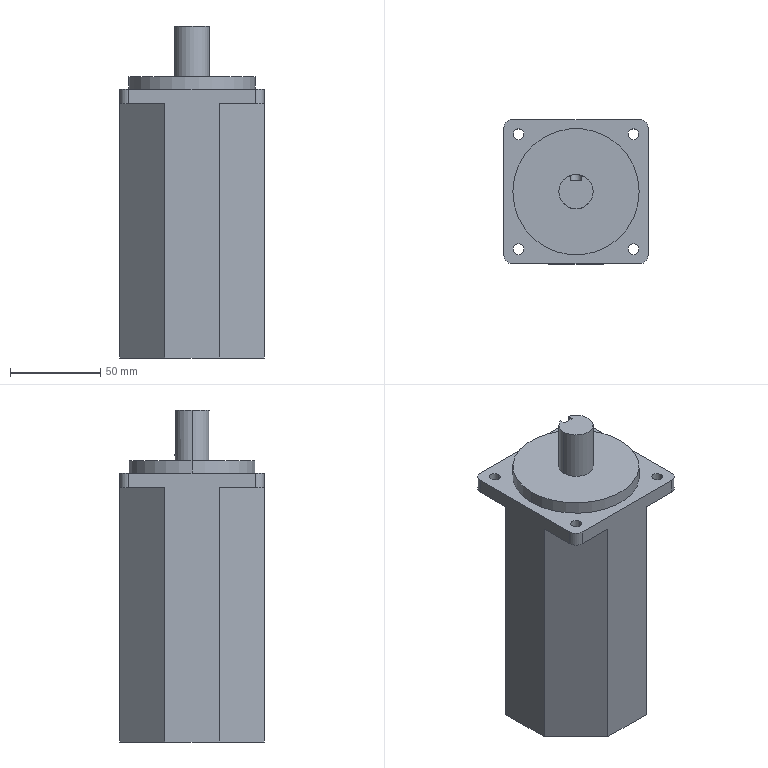Part | SolidWorks | features ICE 6, CombineBodies 1, Extrusion 1, Fillet 1 | 1 solid | 36 faces | box 80 x 80 x 184 mm | volume 810663 mm3 | plane 19 | cylinder 17 | commonest cylinder face diameters 6 x9 10 x4 19 x2 70 x2
STEP:
#1=CARTESIAN_POINT('',(49.5,40.,184.));
#2=VERTEX_POINT('',#1);
#3=CARTESIAN_POINT('',(43.,49.014,184.));
#4=VERTEX_POINT('',#3);
#5=CARTESIAN_POINT('',(40.,40.,184.));
#6=DIRECTION('',(0.,0.,1.));
#7=DIRECTION('',(1.,0.,0.));
#8=AXIS2_PLACEMENT_3D('',#5,#6,#7);
#9=CIRCLE('',#8,9.5);
#10=EDGE_CURVE('',#2,#4,#9,.T.);
#11=ORIENTED_EDGE('',*,*,#10,.F.);
#12=CARTESIAN_POINT('',(49.5,40.,156.));
#13=VERTEX_POINT('',#12);
#14=CARTESIAN_POINT('',(49.5,40.,184.));
#15=DIRECTION('',(0.,0.,-1.));
#16=VECTOR('',#15,1000.);
#17=LINE('',#14,#16);
#18=EDGE_CURVE('',#2,#13,#17,.T.);
#19=ORIENTED_EDGE('',*,*,#18,.T.);
#20=CARTESIAN_POINT('',(30.5,40.,156.));
#21=VERTEX_POINT('',#20);
#22=CARTESIAN_POINT('',(40.,40.,156.));
#23=DIRECTION('',(0.,0.,1.));
#24=DIRECTION('',(1.,0.,0.));
#25=AXIS2_PLACEMENT_3D('',#22,#23,#24);
#26=CIRCLE('',#25,9.5);
#27=EDGE_CURVE('',#13,#21,#26,.T.);
#28=ORIENTED_EDGE('',*,*,#27,.T.);
#29=CARTESIAN_POINT('',(30.5,40.,184.));
#30=VERTEX_POINT('',#29);
#31=CARTESIAN_POINT('',(30.5,40.,184.));
#32=DIRECTION('',(0.,0.,-1.));
#33=VECTOR('',#32,1000.);
#34=LINE('',#31,#33);
#35=EDGE_CURVE('',#30,#21,#34,.T.);
#36=ORIENTED_EDGE('',*,*,#35,.F.);
#37=CARTESIAN_POINT('',(37.,49.014,184.));
#38=VERTEX_POINT('',#37);
#39=CARTESIAN_POINT('',(40.,40.,184.));
#40=DIRECTION('',(0.,0.,1.));
#41=DIRECTION('',(1.,0.,0.));
#42=AXIS2_PLACEMENT_3D('',#39,#40,#41);
#43=CIRCLE('',#42,9.5);
#44=EDGE_CURVE('',#38,#30,#43,.T.);
#45=ORIENTED_EDGE('',*,*,#44,.F.);
#46=CARTESIAN_POINT('',(37.,49.014,162.));
#47=VERTEX_POINT('',#46);
#48=CARTESIAN_POINT('',(37.,49.014,184.));
#49=DIRECTION('',(0.,0.,-1.));
#50=VECTOR('',#49,1000.);
#51=LINE('',#48,#50);
#52=EDGE_CURVE('',#38,#47,#51,.T.);
#53=ORIENTED_EDGE('',*,*,#52,.T.);
#54=CARTESIAN_POINT('',(43.,49.014,162.));
#55=VERTEX_POINT('',#54);
#56=CARTESIAN_POINT('',(37.,49.014,162.));
#57=CARTESIAN_POINT('',(37.,49.014,161.803));
#58=CARTESIAN_POINT('',(37.02,49.021,161.603));
#59=CARTESIAN_POINT('',(37.097,49.046,161.217));
#60=CARTESIAN_POINT('',(37.154,49.064,161.029));
#61=CARTESIAN_POINT('',(37.306,49.11,160.665));
#62=CARTESIAN_POINT('',(37.4,49.138,160.492));
#63=CARTESIAN_POINT('',(37.616,49.197,160.168));
#64=CARTESIAN_POINT('',(37.742,49.229,160.016));
#65=CARTESIAN_POINT('',(38.018,49.292,159.739));
#66=CARTESIAN_POINT('',(38.168,49.323,159.616));
#67=CARTESIAN_POINT('',(38.493,49.381,159.399));
#68=CARTESIAN_POINT('',(38.668,49.408,159.305));
#69=CARTESIAN_POINT('',(39.03,49.452,159.155));
#70=CARTESIAN_POINT('',(39.217,49.47,159.097));
#71=CARTESIAN_POINT('',(39.605,49.494,159.02));
#72=CARTESIAN_POINT('',(39.803,49.5,159.));
#73=CARTESIAN_POINT('',(40.197,49.5,159.));
#74=CARTESIAN_POINT('',(40.394,49.494,159.019));
#75=CARTESIAN_POINT('',(40.784,49.47,159.097));
#76=CARTESIAN_POINT('',(40.971,49.452,159.155));
#77=CARTESIAN_POINT('',(41.333,49.408,159.305));
#78=CARTESIAN_POINT('',(41.508,49.381,159.399));
#79=CARTESIAN_POINT('',(41.833,49.323,159.617));
#80=CARTESIAN_POINT('',(41.983,49.292,159.74));
#81=CARTESIAN_POINT('',(42.26,49.228,160.017));
#82=CARTESIAN_POINT('',(42.385,49.197,160.169));
#83=CARTESIAN_POINT('',(42.601,49.138,160.493));
#84=CARTESIAN_POINT('',(42.694,49.11,160.665));
#85=CARTESIAN_POINT('',(42.846,49.064,161.03));
#86=CARTESIAN_POINT('',(42.903,49.046,161.218));
#87=CARTESIAN_POINT('',(42.98,49.021,161.603));
#88=CARTESIAN_POINT('',(43.,49.014,161.802));
#89=CARTESIAN_POINT('',(43.,49.014,162.));
#90=B_SPLINE_CURVE_WITH_KNOTS('',3,(#56,#57,#58,#59,#60,#61,#62,#63,#64,#65,#66,#67,#68,#69,#70,#71,#72,#73,#74,#75,#76,#77,#78,#79,#80,#81,#82,#83,#84,#85,#86,#87,#88,#89),.UNSPECIFIED.,.F.,.F.,(4,2,2,2,2,2,2,2,2,2,2,2,2,2,2,2,4),(0.004722,0.005311,0.005901,0.006491,0.007081,0.007671,0.008261,0.00885,0.00944,0.01003,0.01062,0.01121,0.0118,0.01239,0.01298,0.01357,0.01416),.UNSPECIFIED.);
#91=EDGE_CURVE('',#47,#55,#90,.T.);
#92=ORIENTED_EDGE('',*,*,#91,.T.);
#93=CARTESIAN_POINT('',(43.,49.014,184.));
#94=DIRECTION('',(0.,0.,1.));
#95=VECTOR('',#94,1000.);
#96=LINE('',#93,#95);
#97=EDGE_CURVE('',#55,#4,#96,.T.);
#98=ORIENTED_EDGE('',*,*,#97,.T.);
#99=EDGE_LOOP('',(#11,#19,#28,#36,#45,#53,#92,#98));
#100=FACE_OUTER_BOUND('',#99,.T.);
#101=CARTESIAN_POINT('',(40.,40.,184.));
#102=DIRECTION('',(0.,0.,-1.));
#103=DIRECTION('',(-1.,0.,0.));
#104=AXIS2_PLACEMENT_3D('',#101,#102,#103);
#105=CYLINDRICAL_SURFACE('',#104,9.5);
#106=ADVANCED_FACE('',(#100),#105,.T.);
#107=CARTESIAN_POINT('',(5.18,8.18,141.));
#108=VERTEX_POINT('',#107);
#109=CARTESIAN_POINT('',(11.18,8.18,141.));
#110=VERTEX_POINT('',#109);
#111=CARTESIAN_POINT('',(8.18,8.18,141.));
#112=DIRECTION('',(0.,0.,1.));
#113=DIRECTION('',(1.,0.,0.));
#114=AXIS2_PLACEMENT_3D('',#111,#112,#113);
#115=CIRCLE('',#114,3.);
#116=EDGE_CURVE('',#108,#110,#115,.T.);
#117=ORIENTED_EDGE('',*,*,#116,.F.);
#118=CARTESIAN_POINT('',(5.18,8.18,149.));
#119=VERTEX_POINT('',#118);
#120=CARTESIAN_POINT('',(5.18,8.18,141.));
#121=DIRECTION('',(0.,0.,1.));
#122=VECTOR('',#121,1000.);
#123=LINE('',#120,#122);
#124=EDGE_CURVE('',#108,#119,#123,.T.);
#125=ORIENTED_EDGE('',*,*,#124,.T.);
#126=CARTESIAN_POINT('',(11.18,8.18,149.));
#127=VERTEX_POINT('',#126);
#128=CARTESIAN_POINT('',(8.18,8.18,149.));
#129=DIRECTION('',(0.,0.,1.));
#130=DIRECTION('',(1.,0.,0.));
#131=AXIS2_PLACEMENT_3D('',#128,#129,#130);
#132=CIRCLE('',#131,3.);
#133=EDGE_CURVE('',#119,#127,#132,.T.);
#134=ORIENTED_EDGE('',*,*,#133,.T.);
#135=CARTESIAN_POINT('',(11.18,8.18,141.));
#136=DIRECTION('',(0.,0.,1.));
#137=VECTOR('',#136,1000.);
#138=LINE('',#135,#137);
#139=EDGE_CURVE('',#110,#127,#138,.T.);
#140=ORIENTED_EDGE('',*,*,#139,.F.);
#141=EDGE_LOOP('',(#117,#125,#134,#140));
#142=FACE_OUTER_BOUND('',#141,.T.);
#143=CARTESIAN_POINT('',(8.18,8.18,141.));
#144=DIRECTION('',(0.,0.,1.));
#145=DIRECTION('',(1.,0.,0.));
#146=AXIS2_PLACEMENT_3D('',#143,#144,#145);
#147=CYLINDRICAL_SURFACE('',#146,3.);
#148=ADVANCED_FACE('',(#142),#147,.F.);
#149=CARTESIAN_POINT('',(68.82,8.18,141.));
#150=VERTEX_POINT('',#149);
#151=CARTESIAN_POINT('',(74.82,8.18,141.));
#152=VERTEX_POINT('',#151);
#153=CARTESIAN_POINT('',(71.82,8.18,141.));
#154=DIRECTION('',(0.,0.,1.));
#155=DIRECTION('',(1.,0.,0.));
#156=AXIS2_PLACEMENT_3D('',#153,#154,#155);
#157=CIRCLE('',#156,3.);
#158=EDGE_CURVE('',#150,#152,#157,.T.);
#159=ORIENTED_EDGE('',*,*,#158,.F.);
#160=CARTESIAN_POINT('',(68.82,8.18,149.));
#161=VERTEX_POINT('',#160);
#162=CARTESIAN_POINT('',(68.82,8.18,141.));
#163=DIRECTION('',(0.,0.,1.));
#164=VECTOR('',#163,1000.);
#165=LINE('',#162,#164);
#166=EDGE_CURVE('',#150,#161,#165,.T.);
#167=ORIENTED_EDGE('',*,*,#166,.T.);
#168=CARTESIAN_POINT('',(74.82,8.18,149.));
#169=VERTEX_POINT('',#168);
#170=CARTESIAN_POINT('',(71.82,8.18,149.));
#171=DIRECTION('',(0.,0.,1.));
#172=DIRECTION('',(1.,0.,0.));
#173=AXIS2_PLACEMENT_3D('',#170,#171,#172);
#174=CIRCLE('',#173,3.);
#175=EDGE_CURVE('',#161,#169,#174,.T.);
#176=ORIENTED_EDGE('',*,*,#175,.T.);
#177=CARTESIAN_POINT('',(74.82,8.18,141.));
#178=DIRECTION('',(0.,0.,1.));
#179=VECTOR('',#178,1000.);
#180=LINE('',#177,#179);
#181=EDGE_CURVE('',#152,#169,#180,.T.);
#182=ORIENTED_EDGE('',*,*,#181,.F.);
#183=EDGE_LOOP('',(#159,#167,#176,#182));
#184=FACE_OUTER_BOUND('',#183,.T.);
#185=CARTESIAN_POINT('',(71.82,8.18,141.));
#186=DIRECTION('',(0.,0.,1.));
#187=DIRECTION('',(1.,0.,0.));
#188=AXIS2_PLACEMENT_3D('',#185,#186,#187);
#189=CYLINDRICAL_SURFACE('',#188,3.);
#190=ADVANCED_FACE('',(#184),#189,.F.);
#191=CARTESIAN_POINT('',(68.82,71.82,141.));
#192=VERTEX_POINT('',#191);
#193=CARTESIAN_POINT('',(74.82,71.82,141.));
#194=VERTEX_POINT('',#193);
#195=CARTESIAN_POINT('',(71.82,71.82,141.));
#196=DIRECTION('',(0.,0.,1.));
#197=DIRECTION('',(1.,0.,0.));
#198=AXIS2_PLACEMENT_3D('',#195,#196,#197);
#199=CIRCLE('',#198,3.);
#200=EDGE_CURVE('',#192,#194,#199,.T.);
#201=ORIENTED_EDGE('',*,*,#200,.F.);
#202=CARTESIAN_POINT('',(68.82,71.82,149.));
#203=VERTEX_POINT('',#202);
#204=CARTESIAN_POINT('',(68.82,71.82,141.));
#205=DIRECTION('',(0.,0.,1.));
#206=VECTOR('',#205,1000.);
#207=LINE('',#204,#206);
#208=EDGE_CURVE('',#192,#203,#207,.T.);
#209=ORIENTED_EDGE('',*,*,#208,.T.);
#210=CARTESIAN_POINT('',(74.82,71.82,149.));
#211=VERTEX_POINT('',#210);
#212=CARTESIAN_POINT('',(71.82,71.82,149.));
#213=DIRECTION('',(0.,0.,1.));
#214=DIRECTION('',(1.,0.,0.));
#215=AXIS2_PLACEMENT_3D('',#212,#213,#214);
#216=CIRCLE('',#215,3.);
#217=EDGE_CURVE('',#203,#211,#216,.T.);
#218=ORIENTED_EDGE('',*,*,#217,.T.);
#219=CARTESIAN_POINT('',(74.82,71.82,141.));
#220=DIRECTION('',(0.,0.,1.));
#221=VECTOR('',#220,1000.);
#222=LINE('',#219,#221);
#223=EDGE_CURVE('',#194,#211,#222,.T.);
#224=ORIENTED_EDGE('',*,*,#223,.F.);
#225=EDGE_LOOP('',(#201,#209,#218,#224));
#226=FACE_OUTER_BOUND('',#225,.T.);
#227=CARTESIAN_POINT('',(71.82,71.82,141.));
#228=DIRECTION('',(0.,0.,1.));
#229=DIRECTION('',(1.,0.,0.));
#230=AXIS2_PLACEMENT_3D('',#227,#228,#229);
#231=CYLINDRICAL_SURFACE('',#230,3.);
#232=ADVANCED_FACE('',(#226),#231,.F.);
#233=CARTESIAN_POINT('',(5.18,71.82,141.));
#234=VERTEX_POINT('',#233);
#235=CARTESIAN_POINT('',(11.18,71.82,141.));
#236=VERTEX_POINT('',#235);
#237=CARTESIAN_POINT('',(8.18,71.82,141.));
#238=DIRECTION('',(0.,0.,1.));
#239=DIRECTION('',(1.,0.,0.));
#240=AXIS2_PLACEMENT_3D('',#237,#238,#239);
#241=CIRCLE('',#240,3.);
#242=EDGE_CURVE('',#234,#236,#241,.T.);
#243=ORIENTED_EDGE('',*,*,#242,.F.);
#244=CARTESIAN_POINT('',(5.18,71.82,149.));
#245=VERTEX_POINT('',#244);
#246=CARTESIAN_POINT('',(5.18,71.82,141.));
#247=DIRECTION('',(0.,0.,1.));
#248=VECTOR('',#247,1000.);
#249=LINE('',#246,#248);
#250=EDGE_CURVE('',#234,#245,#249,.T.);
#251=ORIENTED_EDGE('',*,*,#250,.T.);
#252=CARTESIAN_POINT('',(11.18,71.82,149.));
#253=VERTEX_POINT('',#252);
#254=CARTESIAN_POINT('',(8.18,71.82,149.));
#255=DIRECTION('',(0.,0.,1.));
#256=DIRECTION('',(1.,0.,0.));
#257=AXIS2_PLACEMENT_3D('',#254,#255,#256);
#258=CIRCLE('',#257,3.);
#259=EDGE_CURVE('',#245,#253,#258,.T.);
#260=ORIENTED_EDGE('',*,*,#259,.T.);
#261=CARTESIAN_POINT('',(11.18,71.82,141.));
#262=DIRECTION('',(0.,0.,1.));
#263=VECTOR('',#262,1000.);
#264=LINE('',#261,#263);
#265=EDGE_CURVE('',#236,#253,#264,.T.);
#266=ORIENTED_EDGE('',*,*,#265,.F.);
#267=EDGE_LOOP('',(#243,#251,#260,#266));
#268=FACE_OUTER_BOUND('',#267,.T.);
#269=CARTESIAN_POINT('',(8.18,71.82,141.));
#270=DIRECTION('',(0.,0.,1.));
#271=DIRECTION('',(1.,0.,0.));
#272=AXIS2_PLACEMENT_3D('',#269,#270,#271);
#273=CYLINDRICAL_SURFACE('',#272,3.);
#274=ADVANCED_FACE('',(#268),#273,.F.);
#275=CARTESIAN_POINT('',(75.,40.,156.));
#276=VERTEX_POINT('',#275);
#277=CARTESIAN_POINT('',(5.,40.,156.));
#278=VERTEX_POINT('',#277);
#279=CARTESIAN_POINT('',(40.,40.,156.));
#280=DIRECTION('',(0.,0.,1.));
#281=DIRECTION('',(1.,0.,0.));
#282=AXIS2_PLACEMENT_3D('',#279,#280,#281);
#283=CIRCLE('',#282,35.);
#284=EDGE_CURVE('',#276,#278,#283,.T.);
#285=ORIENTED_EDGE('',*,*,#284,.F.);
#286=CARTESIAN_POINT('',(75.,40.,149.));
#287=VERTEX_POINT('',#286);
#288=CARTESIAN_POINT('',(75.,40.,156.));
#289=DIRECTION('',(0.,0.,-1.));
#290=VECTOR('',#289,1000.);
#291=LINE('',#288,#290);
#292=EDGE_CURVE('',#276,#287,#291,.T.);
#293=ORIENTED_EDGE('',*,*,#292,.T.);
#294=CARTESIAN_POINT('',(5.,40.,149.));
#295=VERTEX_POINT('',#294);
#296=CARTESIAN_POINT('',(40.,40.,149.));
#297=DIRECTION('',(0.,0.,1.));
#298=DIRECTION('',(1.,0.,0.));
#299=AXIS2_PLACEMENT_3D('',#296,#297,#298);
#300=CIRCLE('',#299,35.);
#301=EDGE_CURVE('',#287,#295,#300,.T.);
#302=ORIENTED_EDGE('',*,*,#301,.T.);
#303=CARTESIAN_POINT('',(5.,40.,156.));
#304=DIRECTION('',(0.,0.,-1.));
#305=VECTOR('',#304,1000.);
#306=LINE('',#303,#305);
#307=EDGE_CURVE('',#278,#295,#306,.T.);
#308=ORIENTED_EDGE('',*,*,#307,.F.);
#309=EDGE_LOOP('',(#285,#293,#302,#308));
#310=FACE_OUTER_BOUND('',#309,.T.);
#311=CARTESIAN_POINT('',(40.,40.,156.));
#312=DIRECTION('',(0.,0.,-1.));
#313=DIRECTION('',(-1.,0.,0.));
#314=AXIS2_PLACEMENT_3D('',#311,#312,#313);
#315=CYLINDRICAL_SURFACE('',#314,35.);
#316=ADVANCED_FACE('',(#310),#315,.T.);
#317=CARTESIAN_POINT('',(40.,40.,156.));
#318=DIRECTION('',(0.,0.,1.));
#319=DIRECTION('',(1.,0.,0.));
#320=AXIS2_PLACEMENT_3D('',#317,#318,#319);
#321=CIRCLE('',#320,35.);
#322=EDGE_CURVE('',#278,#276,#321,.T.);
#323=ORIENTED_EDGE('',*,*,#322,.T.);
#324=ORIENTED_EDGE('',*,*,#284,.T.);
#325=EDGE_LOOP('',(#323,#324));
#326=FACE_OUTER_BOUND('',#325,.T.);
#327=CARTESIAN_POINT('',(40.,40.,156.));
#328=DIRECTION('',(0.,0.,1.));
#329=DIRECTION('',(1.,0.,0.));
#330=AXIS2_PLACEMENT_3D('',#327,#328,#329);
#331=CIRCLE('',#330,9.5);
#332=EDGE_CURVE('',#21,#13,#331,.T.);
#333=ORIENTED_EDGE('',*,*,#332,.F.);
#334=ORIENTED_EDGE('',*,*,#27,.F.);
#335=EDGE_LOOP('',(#333,#334));
#336=FACE_BOUND('',#335,.T.);
#337=CARTESIAN_POINT('',(40.,40.,156.));
#338=DIRECTION('',(0.,0.,1.));
#339=DIRECTION('',(1.,0.,0.));
#340=AXIS2_PLACEMENT_3D('',#337,#338,#339);
#341=PLANE('',#340);
#342=ADVANCED_FACE('',(#326,#336),#341,.T.);
#343=CARTESIAN_POINT('',(8.18,8.18,149.));
#344=DIRECTION('',(0.,0.,1.));
#345=DIRECTION('',(1.,0.,0.));
#346=AXIS2_PLACEMENT_3D('',#343,#344,#345);
#347=CIRCLE('',#346,3.);
#348=EDGE_CURVE('',#127,#119,#347,.T.);
#349=ORIENTED_EDGE('',*,*,#348,.F.);
#350=ORIENTED_EDGE('',*,*,#133,.F.);
#351=EDGE_LOOP('',(#349,#350));
#352=FACE_BOUND('',#351,.T.);
#353=CARTESIAN_POINT('',(71.82,8.18,149.));
#354=DIRECTION('',(0.,0.,1.));
#355=DIRECTION('',(1.,0.,0.));
#356=AXIS2_PLACEMENT_3D('',#353,#354,#355);
#357=CIRCLE('',#356,3.);
#358=EDGE_CURVE('',#169,#161,#357,.T.);
#359=ORIENTED_EDGE('',*,*,#358,.F.);
#360=ORIENTED_EDGE('',*,*,#175,.F.);
#361=EDGE_LOOP('',(#359,#360));
#362=FACE_BOUND('',#361,.T.);
#363=CARTESIAN_POINT('',(71.82,71.82,149.));
#364=DIRECTION('',(0.,0.,1.));
#365=DIRECTION('',(1.,0.,0.));
#366=AXIS2_PLACEMENT_3D('',#363,#364,#365);
#367=CIRCLE('',#366,3.);
#368=EDGE_CURVE('',#211,#203,#367,.T.);
#369=ORIENTED_EDGE('',*,*,#368,.F.);
#370=ORIENTED_EDGE('',*,*,#217,.F.);
#371=EDGE_LOOP('',(#369,#370));
#372=FACE_BOUND('',#371,.T.);
#373=CARTESIAN_POINT('',(8.18,71.82,149.));
#374=DIRECTION('',(0.,0.,1.));
#375=DIRECTION('',(1.,0.,0.));
#376=AXIS2_PLACEMENT_3D('',#373,#374,#375);
#377=CIRCLE('',#376,3.);
#378=EDGE_CURVE('',#253,#245,#377,.T.);
#379=ORIENTED_EDGE('',*,*,#378,.F.);
#380=ORIENTED_EDGE('',*,*,#259,.F.);
#381=EDGE_LOOP('',(#379,#380));
#382=FACE_BOUND('',#381,.T.);
#383=CARTESIAN_POINT('',(0.,75.,149.));
#384=VERTEX_POINT('',#383);
#385=CARTESIAN_POINT('',(0.,5.,149.));
#386=VERTEX_POINT('',#385);
#387=CARTESIAN_POINT('',(0.,25.,149.));
#388=DIRECTION('',(0.,-1.,0.));
#389=VECTOR('',#388,1000.);
#390=LINE('',#387,#389);
#391=EDGE_CURVE('',#384,#386,#390,.T.);
#392=ORIENTED_EDGE('',*,*,#391,.T.);
#393=CARTESIAN_POINT('',(5.,0.,149.));
#394=VERTEX_POINT('',#393);
#395=CARTESIAN_POINT('',(5.,5.,149.));
#396=DIRECTION('',(0.,0.,1.));
#397=DIRECTION('',(1.,0.,0.));
#398=AXIS2_PLACEMENT_3D('',#395,#396,#397);
#399=CIRCLE('',#398,5.);
#400=EDGE_CURVE('',#386,#394,#399,.T.);
#401=ORIENTED_EDGE('',*,*,#400,.T.);
#402=CARTESIAN_POINT('',(75.,0.,149.));
#403=VERTEX_POINT('',#402);
#404=CARTESIAN_POINT('',(25.,0.,149.));
#405=DIRECTION('',(1.,0.,0.));
#406=VECTOR('',#405,1000.);
#407=LINE('',#404,#406);
#408=EDGE_CURVE('',#394,#403,#407,.T.);
#409=ORIENTED_EDGE('',*,*,#408,.T.);
#410=CARTESIAN_POINT('',(80.,5.,149.));
#411=VERTEX_POINT('',#410);
#412=CARTESIAN_POINT('',(75.,5.,149.));
#413=DIRECTION('',(0.,0.,1.));
#414=DIRECTION('',(1.,0.,0.));
#415=AXIS2_PLACEMENT_3D('',#412,#413,#414);
#416=CIRCLE('',#415,5.);
#417=EDGE_CURVE('',#403,#411,#416,.T.);
#418=ORIENTED_EDGE('',*,*,#417,.T.);
#419=CARTESIAN_POINT('',(80.,75.,149.));
#420=VERTEX_POINT('',#419);
#421=CARTESIAN_POINT('',(80.,25.,149.));
#422=DIRECTION('',(0.,1.,0.));
#423=VECTOR('',#422,1000.);
#424=LINE('',#421,#423);
#425=EDGE_CURVE('',#411,#420,#424,.T.);
#426=ORIENTED_EDGE('',*,*,#425,.T.);
#427=CARTESIAN_POINT('',(75.,80.,149.));
#428=VERTEX_POINT('',#427);
#429=CARTESIAN_POINT('',(75.,75.,149.));
#430=DIRECTION('',(0.,0.,1.));
#431=DIRECTION('',(1.,0.,0.));
#432=AXIS2_PLACEMENT_3D('',#429,#430,#431);
#433=CIRCLE('',#432,5.);
#434=EDGE_CURVE('',#420,#428,#433,.T.);
#435=ORIENTED_EDGE('',*,*,#434,.T.);
#436=CARTESIAN_POINT('',(5.,80.,149.));
#437=VERTEX_POINT('',#436);
#438=CARTESIAN_POINT('',(25.,80.,149.));
#439=DIRECTION('',(-1.,0.,0.));
#440=VECTOR('',#439,1000.);
#441=LINE('',#438,#440);
#442=EDGE_CURVE('',#428,#437,#441,.T.);
#443=ORIENTED_EDGE('',*,*,#442,.T.);
#444=CARTESIAN_POINT('',(5.,75.,149.));
#445=DIRECTION('',(0.,0.,1.));
#446=DIRECTION('',(1.,0.,0.));
#447=AXIS2_PLACEMENT_3D('',#444,#445,#446);
#448=CIRCLE('',#447,5.);
#449=EDGE_CURVE('',#437,#384,#448,.T.);
#450=ORIENTED_EDGE('',*,*,#449,.T.);
#451=EDGE_LOOP('',(#392,#401,#409,#418,#426,#435,#443,#450));
#452=FACE_OUTER_BOUND('',#451,.T.);
#453=CARTESIAN_POINT('',(40.,40.,149.));
#454=DIRECTION('',(0.,0.,1.));
#455=DIRECTION('',(1.,0.,0.));
#456=AXIS2_PLACEMENT_3D('',#453,#454,#455);
#457=CIRCLE('',#456,35.);
#458=EDGE_CURVE('',#295,#287,#457,.T.);
#459=ORIENTED_EDGE('',*,*,#458,.F.);
#460=ORIENTED_EDGE('',*,*,#301,.F.);
#461=EDGE_LOOP('',(#459,#460));
#462=FACE_BOUND('',#461,.T.);
#463=CARTESIAN_POINT('',(80.,80.,149.));
#464=DIRECTION('',(0.,0.,1.));
#465=DIRECTION('',(1.,0.,0.));
#466=AXIS2_PLACEMENT_3D('',#463,#464,#465);
#467=PLANE('',#466);
#468=ADVANCED_FACE('',(#352,#362,#372,#382,#452,#462),#467,.T.);
#469=ORIENTED_EDGE('',*,*,#442,.F.);
#470=CARTESIAN_POINT('',(75.,80.,141.));
#471=VERTEX_POINT('',#470);
#472=CARTESIAN_POINT('',(75.,80.,149.));
#473=DIRECTION('',(0.,0.,-1.));
#474=VECTOR('',#473,1000.);
#475=LINE('',#472,#474);
#476=EDGE_CURVE('',#428,#471,#475,.T.);
#477=ORIENTED_EDGE('',*,*,#476,.T.);
#478=CARTESIAN_POINT('',(55.,80.,141.));
#479=VERTEX_POINT('',#478);
#480=CARTESIAN_POINT('',(0.,80.,141.));
#481=DIRECTION('',(-1.,0.,0.));
#482=VECTOR('',#481,1000.);
#483=LINE('',#480,#482);
#484=EDGE_CURVE('',#471,#479,#483,.T.);
#485=ORIENTED_EDGE('',*,*,#484,.T.);
#486=CARTESIAN_POINT('',(55.,80.,0.));
#487=VERTEX_POINT('',#486);
#488=CARTESIAN_POINT('',(55.,80.,149.));
#489=DIRECTION('',(0.,0.,-1.));
#490=VECTOR('',#489,1000.);
#491=LINE('',#488,#490);
#492=EDGE_CURVE('',#479,#487,#491,.T.);
#493=ORIENTED_EDGE('',*,*,#492,.T.);
#494=CARTESIAN_POINT('',(25.,80.,0.));
#495=VERTEX_POINT('',#494);
#496=CARTESIAN_POINT('',(25.,80.,0.));
#497=DIRECTION('',(-1.,0.,0.));
#498=VECTOR('',#497,1000.);
#499=LINE('',#496,#498);
#500=EDGE_CURVE('',#487,#495,#499,.T.);
#501=ORIENTED_EDGE('',*,*,#500,.T.);
#502=CARTESIAN_POINT('',(25.,80.,141.));
#503=VERTEX_POINT('',#502);
#504=CARTESIAN_POINT('',(25.,80.,149.));
#505=DIRECTION('',(0.,0.,-1.));
#506=VECTOR('',#505,1000.);
#507=LINE('',#504,#506);
#508=EDGE_CURVE('',#503,#495,#507,.T.);
#509=ORIENTED_EDGE('',*,*,#508,.F.);
#510=CARTESIAN_POINT('',(5.,80.,141.));
#511=VERTEX_POINT('',#510);
#512=CARTESIAN_POINT('',(0.,80.,141.));
#513=DIRECTION('',(-1.,0.,0.));
#514=VECTOR('',#513,1000.);
#515=LINE('',#512,#514);
#516=EDGE_CURVE('',#503,#511,#515,.T.);
#517=ORIENTED_EDGE('',*,*,#516,.T.);
#518=CARTESIAN_POINT('',(5.,80.,149.));
#519=DIRECTION('',(0.,0.,1.));
#520=VECTOR('',#519,1000.);
#521=LINE('',#518,#520);
#522=EDGE_CURVE('',#511,#437,#521,.T.);
#523=ORIENTED_EDGE('',*,*,#522,.T.);
#524=EDGE_LOOP('',(#469,#477,#485,#493,#501,#509,#517,#523));
#525=FACE_OUTER_BOUND('',#524,.T.);
#526=CARTESIAN_POINT('',(25.,80.,149.));
#527=DIRECTION('',(0.,-1.,0.));
#528=DIRECTION('',(0.,0.,-1.));
#529=AXIS2_PLACEMENT_3D('',#526,#527,#528);
#530=PLANE('',#529);
#531=ADVANCED_FACE('',(#525),#530,.F.);
#532=CARTESIAN_POINT('',(0.,55.,141.));
#533=VERTEX_POINT('',#532);
#534=CARTESIAN_POINT('',(0.,55.,0.));
#535=VERTEX_POINT('',#534);
#536=CARTESIAN_POINT('',(0.,55.,149.));
#537=DIRECTION('',(0.,0.,-1.));
#538=VECTOR('',#537,1000.);
#539=LINE('',#536,#538);
#540=EDGE_CURVE('',#533,#535,#539,.T.);
#541=ORIENTED_EDGE('',*,*,#540,.F.);
#542=CARTESIAN_POINT('',(25.,80.,141.));
#543=DIRECTION('',(0.7071,0.7071,0.));
#544=VECTOR('',#543,1000.);
#545=LINE('',#542,#544);
#546=EDGE_CURVE('',#533,#503,#545,.T.);
#547=ORIENTED_EDGE('',*,*,#546,.T.);
#548=ORIENTED_EDGE('',*,*,#508,.T.);
#549=CARTESIAN_POINT('',(25.,80.,0.));
#550=DIRECTION('',(-0.7071,-0.7071,0.));
#551=VECTOR('',#550,1000.);
#552=LINE('',#549,#551);
#553=EDGE_CURVE('',#495,#535,#552,.T.);
#554=ORIENTED_EDGE('',*,*,#553,.T.);
#555=EDGE_LOOP('',(#541,#547,#548,#554));
#556=FACE_OUTER_BOUND('',#555,.T.);
#557=CARTESIAN_POINT('',(25.,80.,149.));
#558=DIRECTION('',(0.7071,-0.7071,0.));
#559=DIRECTION('',(0.7071,0.7071,0.));
#560=AXIS2_PLACEMENT_3D('',#557,#558,#559);
#561=PLANE('',#560);
#562=ADVANCED_FACE('',(#556),#561,.F.);
#563=CARTESIAN_POINT('',(0.,25.,141.));
#564=VERTEX_POINT('',#563);
#565=CARTESIAN_POINT('',(0.,5.,141.));
#566=VERTEX_POINT('',#565);
#567=CARTESIAN_POINT('',(0.,0.,141.));
#568=DIRECTION('',(0.,-1.,0.));
#569=VECTOR('',#568,1000.);
#570=LINE('',#567,#569);
#571=EDGE_CURVE('',#564,#566,#570,.T.);
#572=ORIENTED_EDGE('',*,*,#571,.T.);
#573=CARTESIAN_POINT('',(0.,5.,149.));
#574=DIRECTION('',(0.,0.,1.));
#575=VECTOR('',#574,1000.);
#576=LINE('',#573,#575);
#577=EDGE_CURVE('',#566,#386,#576,.T.);
#578=ORIENTED_EDGE('',*,*,#577,.T.);
#579=ORIENTED_EDGE('',*,*,#391,.F.);
#580=CARTESIAN_POINT('',(0.,75.,141.));
#581=VERTEX_POINT('',#580);
#582=CARTESIAN_POINT('',(0.,75.,149.));
#583=DIRECTION('',(0.,0.,-1.));
#584=VECTOR('',#583,1000.);
#585=LINE('',#582,#584);
#586=EDGE_CURVE('',#384,#581,#585,.T.);
#587=ORIENTED_EDGE('',*,*,#586,.T.);
#588=CARTESIAN_POINT('',(0.,0.,141.));
#589=DIRECTION('',(0.,-1.,0.));
#590=VECTOR('',#589,1000.);
#591=LINE('',#588,#590);
#592=EDGE_CURVE('',#581,#533,#591,.T.);
#593=ORIENTED_EDGE('',*,*,#592,.T.);
#594=ORIENTED_EDGE('',*,*,#540,.T.);
#595=CARTESIAN_POINT('',(0.,25.,0.));
#596=VERTEX_POINT('',#595);
#597=CARTESIAN_POINT('',(0.,25.,0.));
#598=DIRECTION('',(0.,-1.,0.));
#599=VECTOR('',#598,1000.);
#600=LINE('',#597,#599);
#601=EDGE_CURVE('',#535,#596,#600,.T.);
#602=ORIENTED_EDGE('',*,*,#601,.T.);
#603=CARTESIAN_POINT('',(0.,25.,149.));
#604=DIRECTION('',(0.,0.,-1.));
#605=VECTOR('',#604,1000.);
#606=LINE('',#603,#605);
#607=EDGE_CURVE('',#564,#596,#606,.T.);
#608=ORIENTED_EDGE('',*,*,#607,.F.);
#609=EDGE_LOOP('',(#572,#578,#579,#587,#593,#594,#602,#608));
#610=FACE_OUTER_BOUND('',#609,.T.);
#611=CARTESIAN_POINT('',(0.,25.,149.));
#612=DIRECTION('',(1.,0.,0.));
#613=DIRECTION('',(0.,1.,0.));
#614=AXIS2_PLACEMENT_3D('',#611,#612,#613);
#615=PLANE('',#614);
#616=ADVANCED_FACE('',(#610),#615,.F.);
#617=CARTESIAN_POINT('',(25.,0.,141.));
#618=VERTEX_POINT('',#617);
#619=CARTESIAN_POINT('',(25.,0.,0.));
#620=VERTEX_POINT('',#619);
#621=CARTESIAN_POINT('',(25.,0.,149.));
#622=DIRECTION('',(0.,0.,-1.));
#623=VECTOR('',#622,1000.);
#624=LINE('',#621,#623);
#625=EDGE_CURVE('',#618,#620,#624,.T.);
#626=ORIENTED_EDGE('',*,*,#625,.F.);
#627=CARTESIAN_POINT('',(0.,25.,141.));
#628=DIRECTION('',(-0.7071,0.7071,0.));
#629=VECTOR('',#628,1000.);
#630=LINE('',#627,#629);
#631=EDGE_CURVE('',#618,#564,#630,.T.);
#632=ORIENTED_EDGE('',*,*,#631,.T.);
#633=ORIENTED_EDGE('',*,*,#607,.T.);
#634=CARTESIAN_POINT('',(0.,25.,0.));
#635=DIRECTION('',(0.7071,-0.7071,0.));
#636=VECTOR('',#635,1000.);
#637=LINE('',#634,#636);
#638=EDGE_CURVE('',#596,#620,#637,.T.);
#639=ORIENTED_EDGE('',*,*,#638,.T.);
#640=EDGE_LOOP('',(#626,#632,#633,#639));
#641=FACE_OUTER_BOUND('',#640,.T.);
#642=CARTESIAN_POINT('',(0.,25.,149.));
#643=DIRECTION('',(0.7071,0.7071,0.));
#644=DIRECTION('',(-0.7071,0.7071,0.));
#645=AXIS2_PLACEMENT_3D('',#642,#643,#644);
#646=PLANE('',#645);
#647=ADVANCED_FACE('',(#641),#646,.F.);
#648=ORIENTED_EDGE('',*,*,#408,.F.);
#649=CARTESIAN_POINT('',(5.,0.,141.));
#650=VERTEX_POINT('',#649);
#651=CARTESIAN_POINT('',(5.,0.,149.));
#652=DIRECTION('',(0.,0.,-1.));
#653=VECTOR('',#652,1000.);
#654=LINE('',#651,#653);
#655=EDGE_CURVE('',#394,#650,#654,.T.);
#656=ORIENTED_EDGE('',*,*,#655,.T.);
#657=CARTESIAN_POINT('',(0.,0.,141.));
#658=DIRECTION('',(1.,0.,0.));
#659=VECTOR('',#658,1000.);
#660=LINE('',#657,#659);
#661=EDGE_CURVE('',#650,#618,#660,.T.);
#662=ORIENTED_EDGE('',*,*,#661,.T.);
#663=ORIENTED_EDGE('',*,*,#625,.T.);
#664=CARTESIAN_POINT('',(55.,0.,0.));
#665=VERTEX_POINT('',#664);
#666=CARTESIAN_POINT('',(25.,0.,0.));
#667=DIRECTION('',(1.,0.,0.));
#668=VECTOR('',#667,1000.);
#669=LINE('',#666,#668);
#670=EDGE_CURVE('',#620,#665,#669,.T.);
#671=ORIENTED_EDGE('',*,*,#670,.T.);
#672=CARTESIAN_POINT('',(55.,0.,141.));
#673=VERTEX_POINT('',#672);
#674=CARTESIAN_POINT('',(55.,0.,149.));
#675=DIRECTION('',(0.,0.,-1.));
#676=VECTOR('',#675,1000.);
#677=LINE('',#674,#676);
#678=EDGE_CURVE('',#673,#665,#677,.T.);
#679=ORIENTED_EDGE('',*,*,#678,.F.);
#680=CARTESIAN_POINT('',(75.,0.,141.));
#681=VERTEX_POINT('',#680);
#682=CARTESIAN_POINT('',(0.,0.,141.));
#683=DIRECTION('',(1.,0.,0.));
#684=VECTOR('',#683,1000.);
#685=LINE('',#682,#684);
#686=EDGE_CURVE('',#673,#681,#685,.T.);
#687=ORIENTED_EDGE('',*,*,#686,.T.);
#688=CARTESIAN_POINT('',(75.,0.,149.));
#689=DIRECTION('',(0.,0.,1.));
#690=VECTOR('',#689,1000.);
#691=LINE('',#688,#690);
#692=EDGE_CURVE('',#681,#403,#691,.T.);
#693=ORIENTED_EDGE('',*,*,#692,.T.);
#694=EDGE_LOOP('',(#648,#656,#662,#663,#671,#679,#687,#693));
#695=FACE_OUTER_BOUND('',#694,.T.);
#696=CARTESIAN_POINT('',(25.,0.,149.));
#697=DIRECTION('',(0.,1.,0.));
#698=DIRECTION('',(0.,0.,1.));
#699=AXIS2_PLACEMENT_3D('',#696,#697,#698);
#700=PLANE('',#699);
#701=ADVANCED_FACE('',(#695),#700,.F.);
#702=CARTESIAN_POINT('',(80.,25.,141.));
#703=VERTEX_POINT('',#702);
#704=CARTESIAN_POINT('',(80.,25.,0.));
#705=VERTEX_POINT('',#704);
#706=CARTESIAN_POINT('',(80.,25.,149.));
#707=DIRECTION('',(0.,0.,-1.));
#708=VECTOR('',#707,1000.);
#709=LINE('',#706,#708);
#710=EDGE_CURVE('',#703,#705,#709,.T.);
#711=ORIENTED_EDGE('',*,*,#710,.F.);
#712=CARTESIAN_POINT('',(80.,25.,141.));
#713=DIRECTION('',(-0.7071,-0.7071,0.));
#714=VECTOR('',#713,1000.);
#715=LINE('',#712,#714);
#716=EDGE_CURVE('',#703,#673,#715,.T.);
#717=ORIENTED_EDGE('',*,*,#716,.T.);
#718=ORIENTED_EDGE('',*,*,#678,.T.);
#719=CARTESIAN_POINT('',(80.,25.,0.));
#720=DIRECTION('',(0.7071,0.7071,0.));
#721=VECTOR('',#720,1000.);
#722=LINE('',#719,#721);
#723=EDGE_CURVE('',#665,#705,#722,.T.);
#724=ORIENTED_EDGE('',*,*,#723,.T.);
#725=EDGE_LOOP('',(#711,#717,#718,#724));
#726=FACE_OUTER_BOUND('',#725,.T.);
#727=CARTESIAN_POINT('',(80.,25.,149.));
#728=DIRECTION('',(-0.7071,0.7071,0.));
#729=DIRECTION('',(-0.7071,-0.7071,0.));
#730=AXIS2_PLACEMENT_3D('',#727,#728,#729);
#731=PLANE('',#730);
#732=ADVANCED_FACE('',(#726),#731,.F.);
#733=ORIENTED_EDGE('',*,*,#425,.F.);
#734=CARTESIAN_POINT('',(80.,5.,141.));
#735=VERTEX_POINT('',#734);
#736=CARTESIAN_POINT('',(80.,5.,149.));
#737=DIRECTION('',(0.,0.,-1.));
#738=VECTOR('',#737,1000.);
#739=LINE('',#736,#738);
#740=EDGE_CURVE('',#411,#735,#739,.T.);
#741=ORIENTED_EDGE('',*,*,#740,.T.);
#742=CARTESIAN_POINT('',(80.,0.,141.));
#743=DIRECTION('',(0.,1.,0.));
#744=VECTOR('',#743,1000.);
#745=LINE('',#742,#744);
#746=EDGE_CURVE('',#735,#703,#745,.T.);
#747=ORIENTED_EDGE('',*,*,#746,.T.);
#748=ORIENTED_EDGE('',*,*,#710,.T.);
#749=CARTESIAN_POINT('',(80.,55.,0.));
#750=VERTEX_POINT('',#749);
#751=CARTESIAN_POINT('',(80.,25.,0.));
#752=DIRECTION('',(0.,1.,0.));
#753=VECTOR('',#752,1000.);
#754=LINE('',#751,#753);
#755=EDGE_CURVE('',#705,#750,#754,.T.);
#756=ORIENTED_EDGE('',*,*,#755,.T.);
#757=CARTESIAN_POINT('',(80.,55.,141.));
#758=VERTEX_POINT('',#757);
#759=CARTESIAN_POINT('',(80.,55.,149.));
#760=DIRECTION('',(0.,0.,-1.));
#761=VECTOR('',#760,1000.);
#762=LINE('',#759,#761);
#763=EDGE_CURVE('',#758,#750,#762,.T.);
#764=ORIENTED_EDGE('',*,*,#763,.F.);
#765=CARTESIAN_POINT('',(80.,75.,141.));
#766=VERTEX_POINT('',#765);
#767=CARTESIAN_POINT('',(80.,0.,141.));
#768=DIRECTION('',(0.,1.,0.));
#769=VECTOR('',#768,1000.);
#770=LINE('',#767,#769);
#771=EDGE_CURVE('',#758,#766,#770,.T.);
#772=ORIENTED_EDGE('',*,*,#771,.T.);
#773=CARTESIAN_POINT('',(80.,75.,149.));
#774=DIRECTION('',(0.,0.,1.));
#775=VECTOR('',#774,1000.);
#776=LINE('',#773,#775);
#777=EDGE_CURVE('',#766,#420,#776,.T.);
#778=ORIENTED_EDGE('',*,*,#777,.T.);
#779=EDGE_LOOP('',(#733,#741,#747,#748,#756,#764,#772,#778));
#780=FACE_OUTER_BOUND('',#779,.T.);
#781=CARTESIAN_POINT('',(80.,25.,149.));
#782=DIRECTION('',(-1.,0.,0.));
#783=DIRECTION('',(0.,-1.,0.));
#784=AXIS2_PLACEMENT_3D('',#781,#782,#783);
#785=PLANE('',#784);
#786=ADVANCED_FACE('',(#780),#785,.F.);
#787=ORIENTED_EDGE('',*,*,#492,.F.);
#788=CARTESIAN_POINT('',(55.,80.,141.));
#789=DIRECTION('',(0.7071,-0.7071,0.));
#790=VECTOR('',#789,1000.);
#791=LINE('',#788,#790);
#792=EDGE_CURVE('',#479,#758,#791,.T.);
#793=ORIENTED_EDGE('',*,*,#792,.T.);
#794=ORIENTED_EDGE('',*,*,#763,.T.);
#795=CARTESIAN_POINT('',(55.,80.,0.));
#796=DIRECTION('',(-0.7071,0.7071,0.));
#797=VECTOR('',#796,1000.);
#798=LINE('',#795,#797);
#799=EDGE_CURVE('',#750,#487,#798,.T.);
#800=ORIENTED_EDGE('',*,*,#799,.T.);
#801=EDGE_LOOP('',(#787,#793,#794,#800));
#802=FACE_OUTER_BOUND('',#801,.T.);
#803=CARTESIAN_POINT('',(55.,80.,149.));
#804=DIRECTION('',(-0.7071,-0.7071,0.));
#805=DIRECTION('',(0.7071,-0.7071,0.));
#806=AXIS2_PLACEMENT_3D('',#803,#804,#805);
#807=PLANE('',#806);
#808=ADVANCED_FACE('',(#802),#807,.F.);
#809=ORIENTED_EDGE('',*,*,#500,.F.);
#810=ORIENTED_EDGE('',*,*,#799,.F.);
#811=ORIENTED_EDGE('',*,*,#755,.F.);
#812=ORIENTED_EDGE('',*,*,#723,.F.);
#813=ORIENTED_EDGE('',*,*,#670,.F.);
#814=ORIENTED_EDGE('',*,*,#638,.F.);
#815=ORIENTED_EDGE('',*,*,#601,.F.);
#816=ORIENTED_EDGE('',*,*,#553,.F.);
#817=EDGE_LOOP('',(#809,#810,#811,#812,#813,#814,#815,#816));
#818=FACE_OUTER_BOUND('',#817,.T.);
#819=CARTESIAN_POINT('',(80.,80.,0.));
#820=DIRECTION('',(0.,0.,1.));
#821=DIRECTION('',(1.,0.,0.));
#822=AXIS2_PLACEMENT_3D('',#819,#820,#821);
#823=PLANE('',#822);
#824=ADVANCED_FACE('',(#818),#823,.F.);
#825=ORIENTED_EDGE('',*,*,#292,.F.);
#826=ORIENTED_EDGE('',*,*,#322,.F.);
#827=ORIENTED_EDGE('',*,*,#307,.T.);
#828=ORIENTED_EDGE('',*,*,#458,.T.);
#829=EDGE_LOOP('',(#825,#826,#827,#828));
#830=FACE_OUTER_BOUND('',#829,.T.);
#831=CARTESIAN_POINT('',(40.,40.,156.));
#832=DIRECTION('',(0.,0.,-1.));
#833=DIRECTION('',(-1.,0.,0.));
#834=AXIS2_PLACEMENT_3D('',#831,#832,#833);
#835=CYLINDRICAL_SURFACE('',#834,35.);
#836=ADVANCED_FACE('',(#830),#835,.T.);
#837=CARTESIAN_POINT('',(71.82,71.82,141.));
#838=DIRECTION('',(0.,0.,1.));
#839=DIRECTION('',(1.,0.,0.));
#840=AXIS2_PLACEMENT_3D('',#837,#838,#839);
#841=CIRCLE('',#840,3.);
#842=EDGE_CURVE('',#194,#192,#841,.T.);
#843=ORIENTED_EDGE('',*,*,#842,.T.);
#844=ORIENTED_EDGE('',*,*,#200,.T.);
#845=EDGE_LOOP('',(#843,#844));
#846=FACE_BOUND('',#845,.T.);
#847=ORIENTED_EDGE('',*,*,#484,.F.);
#848=CARTESIAN_POINT('',(75.,75.,141.));
#849=DIRECTION('',(0.,0.,-1.));
#850=DIRECTION('',(-1.,0.,0.));
#851=AXIS2_PLACEMENT_3D('',#848,#849,#850);
#852=CIRCLE('',#851,5.);
#853=EDGE_CURVE('',#471,#766,#852,.T.);
#854=ORIENTED_EDGE('',*,*,#853,.T.);
#855=ORIENTED_EDGE('',*,*,#771,.F.);
#856=ORIENTED_EDGE('',*,*,#792,.F.);
#857=EDGE_LOOP('',(#847,#854,#855,#856));
#858=FACE_OUTER_BOUND('',#857,.T.);
#859=CARTESIAN_POINT('',(0.,80.,141.));
#860=DIRECTION('',(0.,0.,-1.));
#861=DIRECTION('',(-1.,0.,0.));
#862=AXIS2_PLACEMENT_3D('',#859,#860,#861);
#863=PLANE('',#862);
#864=ADVANCED_FACE('',(#846,#858),#863,.T.);
#865=CARTESIAN_POINT('',(71.82,8.18,141.));
#866=DIRECTION('',(0.,0.,1.));
#867=DIRECTION('',(1.,0.,0.));
#868=AXIS2_PLACEMENT_3D('',#865,#866,#867);
#869=CIRCLE('',#868,3.);
#870=EDGE_CURVE('',#152,#150,#869,.T.);
#871=ORIENTED_EDGE('',*,*,#870,.T.);
#872=ORIENTED_EDGE('',*,*,#158,.T.);
#873=EDGE_LOOP('',(#871,#872));
#874=FACE_BOUND('',#873,.T.);
#875=ORIENTED_EDGE('',*,*,#746,.F.);
#876=CARTESIAN_POINT('',(75.,5.,141.));
#877=DIRECTION('',(0.,0.,-1.));
#878=DIRECTION('',(-1.,0.,0.));
#879=AXIS2_PLACEMENT_3D('',#876,#877,#878);
#880=CIRCLE('',#879,5.);
#881=EDGE_CURVE('',#735,#681,#880,.T.);
#882=ORIENTED_EDGE('',*,*,#881,.T.);
#883=ORIENTED_EDGE('',*,*,#686,.F.);
#884=ORIENTED_EDGE('',*,*,#716,.F.);
#885=EDGE_LOOP('',(#875,#882,#883,#884));
#886=FACE_OUTER_BOUND('',#885,.T.);
#887=CARTESIAN_POINT('',(0.,80.,141.));
#888=DIRECTION('',(0.,0.,-1.));
#889=DIRECTION('',(-1.,0.,0.));
#890=AXIS2_PLACEMENT_3D('',#887,#888,#889);
#891=PLANE('',#890);
#892=ADVANCED_FACE('',(#874,#886),#891,.T.);
#893=CARTESIAN_POINT('',(8.18,8.18,141.));
#894=DIRECTION('',(0.,0.,1.));
#895=DIRECTION('',(1.,0.,0.));
#896=AXIS2_PLACEMENT_3D('',#893,#894,#895);
#897=CIRCLE('',#896,3.);
#898=EDGE_CURVE('',#110,#108,#897,.T.);
#899=ORIENTED_EDGE('',*,*,#898,.T.);
#900=ORIENTED_EDGE('',*,*,#116,.T.);
#901=EDGE_LOOP('',(#899,#900));
#902=FACE_BOUND('',#901,.T.);
#903=ORIENTED_EDGE('',*,*,#661,.F.);
#904=CARTESIAN_POINT('',(5.,5.,141.));
#905=DIRECTION('',(0.,0.,-1.));
#906=DIRECTION('',(-1.,0.,0.));
#907=AXIS2_PLACEMENT_3D('',#904,#905,#906);
#908=CIRCLE('',#907,5.);
#909=EDGE_CURVE('',#650,#566,#908,.T.);
#910=ORIENTED_EDGE('',*,*,#909,.T.);
#911=ORIENTED_EDGE('',*,*,#571,.F.);
#912=ORIENTED_EDGE('',*,*,#631,.F.);
#913=EDGE_LOOP('',(#903,#910,#911,#912));
#914=FACE_OUTER_BOUND('',#913,.T.);
#915=CARTESIAN_POINT('',(0.,80.,141.));
#916=DIRECTION('',(0.,0.,-1.));
#917=DIRECTION('',(-1.,0.,0.));
#918=AXIS2_PLACEMENT_3D('',#915,#916,#917);
#919=PLANE('',#918);
#920=ADVANCED_FACE('',(#902,#914),#919,.T.);
#921=CARTESIAN_POINT('',(8.18,71.82,141.));
#922=DIRECTION('',(0.,0.,1.));
#923=DIRECTION('',(1.,0.,0.));
#924=AXIS2_PLACEMENT_3D('',#921,#922,#923);
#925=CIRCLE('',#924,3.);
#926=EDGE_CURVE('',#236,#234,#925,.T.);
#927=ORIENTED_EDGE('',*,*,#926,.T.);
#928=ORIENTED_EDGE('',*,*,#242,.T.);
#929=EDGE_LOOP('',(#927,#928));
#930=FACE_BOUND('',#929,.T.);
#931=ORIENTED_EDGE('',*,*,#592,.F.);
#932=CARTESIAN_POINT('',(5.,75.,141.));
#933=DIRECTION('',(0.,0.,-1.));
#934=DIRECTION('',(-1.,0.,0.));
#935=AXIS2_PLACEMENT_3D('',#932,#933,#934);
#936=CIRCLE('',#935,5.);
#937=EDGE_CURVE('',#581,#511,#936,.T.);
#938=ORIENTED_EDGE('',*,*,#937,.T.);
#939=ORIENTED_EDGE('',*,*,#516,.F.);
#940=ORIENTED_EDGE('',*,*,#546,.F.);
#941=EDGE_LOOP('',(#931,#938,#939,#940));
#942=FACE_OUTER_BOUND('',#941,.T.);
#943=CARTESIAN_POINT('',(0.,80.,141.));
#944=DIRECTION('',(0.,0.,-1.));
#945=DIRECTION('',(-1.,0.,0.));
#946=AXIS2_PLACEMENT_3D('',#943,#944,#945);
#947=PLANE('',#946);
#948=ADVANCED_FACE('',(#930,#942),#947,.T.);
#949=ORIENTED_EDGE('',*,*,#250,.F.);
#950=ORIENTED_EDGE('',*,*,#926,.F.);
#951=ORIENTED_EDGE('',*,*,#265,.T.);
#952=ORIENTED_EDGE('',*,*,#378,.T.);
#953=EDGE_LOOP('',(#949,#950,#951,#952));
#954=FACE_OUTER_BOUND('',#953,.T.);
#955=CARTESIAN_POINT('',(8.18,71.82,141.));
#956=DIRECTION('',(0.,0.,1.));
#957=DIRECTION('',(1.,0.,0.));
#958=AXIS2_PLACEMENT_3D('',#955,#956,#957);
#959=CYLINDRICAL_SURFACE('',#958,3.);
#960=ADVANCED_FACE('',(#954),#959,.F.);
#961=ORIENTED_EDGE('',*,*,#208,.F.);
#962=ORIENTED_EDGE('',*,*,#842,.F.);
#963=ORIENTED_EDGE('',*,*,#223,.T.);
#964=ORIENTED_EDGE('',*,*,#368,.T.);
#965=EDGE_LOOP('',(#961,#962,#963,#964));
#966=FACE_OUTER_BOUND('',#965,.T.);
#967=CARTESIAN_POINT('',(71.82,71.82,141.));
#968=DIRECTION('',(0.,0.,1.));
#969=DIRECTION('',(1.,0.,0.));
#970=AXIS2_PLACEMENT_3D('',#967,#968,#969);
#971=CYLINDRICAL_SURFACE('',#970,3.);
#972=ADVANCED_FACE('',(#966),#971,.F.);
#973=ORIENTED_EDGE('',*,*,#166,.F.);
#974=ORIENTED_EDGE('',*,*,#870,.F.);
#975=ORIENTED_EDGE('',*,*,#181,.T.);
#976=ORIENTED_EDGE('',*,*,#358,.T.);
#977=EDGE_LOOP('',(#973,#974,#975,#976));
#978=FACE_OUTER_BOUND('',#977,.T.);
#979=CARTESIAN_POINT('',(71.82,8.18,141.));
#980=DIRECTION('',(0.,0.,1.));
#981=DIRECTION('',(1.,0.,0.));
#982=AXIS2_PLACEMENT_3D('',#979,#980,#981);
#983=CYLINDRICAL_SURFACE('',#982,3.);
#984=ADVANCED_FACE('',(#978),#983,.F.);
#985=ORIENTED_EDGE('',*,*,#124,.F.);
#986=ORIENTED_EDGE('',*,*,#898,.F.);
#987=ORIENTED_EDGE('',*,*,#139,.T.);
#988=ORIENTED_EDGE('',*,*,#348,.T.);
#989=EDGE_LOOP('',(#985,#986,#987,#988));
#990=FACE_OUTER_BOUND('',#989,.T.);
#991=CARTESIAN_POINT('',(8.18,8.18,141.));
#992=DIRECTION('',(0.,0.,1.));
#993=DIRECTION('',(1.,0.,0.));
#994=AXIS2_PLACEMENT_3D('',#991,#992,#993);
#995=CYLINDRICAL_SURFACE('',#994,3.);
#996=ADVANCED_FACE('',(#990),#995,.F.);
#997=ORIENTED_EDGE('',*,*,#909,.F.);
#998=ORIENTED_EDGE('',*,*,#655,.F.);
#999=ORIENTED_EDGE('',*,*,#400,.F.);
#1000=ORIENTED_EDGE('',*,*,#577,.F.);
#1001=EDGE_LOOP('',(#997,#998,#999,#1000));
#1002=FACE_OUTER_BOUND('',#1001,.T.);
#1003=CARTESIAN_POINT('',(5.,5.,149.));
#1004=DIRECTION('',(0.,0.,1.));
#1005=DIRECTION('',(1.,0.,0.));
#1006=AXIS2_PLACEMENT_3D('',#1003,#1004,#1005);
#1007=CYLINDRICAL_SURFACE('',#1006,5.);
#1008=ADVANCED_FACE('',(#1002),#1007,.T.);
#1009=ORIENTED_EDGE('',*,*,#881,.F.);
#1010=ORIENTED_EDGE('',*,*,#740,.F.);
#1011=ORIENTED_EDGE('',*,*,#417,.F.);
#1012=ORIENTED_EDGE('',*,*,#692,.F.);
#1013=EDGE_LOOP('',(#1009,#1010,#1011,#1012));
#1014=FACE_OUTER_BOUND('',#1013,.T.);
#1015=CARTESIAN_POINT('',(75.,5.,149.));
#1016=DIRECTION('',(0.,0.,1.));
#1017=DIRECTION('',(1.,0.,0.));
#1018=AXIS2_PLACEMENT_3D('',#1015,#1016,#1017);
#1019=CYLINDRICAL_SURFACE('',#1018,5.);
#1020=ADVANCED_FACE('',(#1014),#1019,.T.);
#1021=ORIENTED_EDGE('',*,*,#853,.F.);
#1022=ORIENTED_EDGE('',*,*,#476,.F.);
#1023=ORIENTED_EDGE('',*,*,#434,.F.);
#1024=ORIENTED_EDGE('',*,*,#777,.F.);
#1025=EDGE_LOOP('',(#1021,#1022,#1023,#1024));
#1026=FACE_OUTER_BOUND('',#1025,.T.);
#1027=CARTESIAN_POINT('',(75.,75.,149.));
#1028=DIRECTION('',(0.,0.,1.));
#1029=DIRECTION('',(1.,0.,0.));
#1030=AXIS2_PLACEMENT_3D('',#1027,#1028,#1029);
#1031=CYLINDRICAL_SURFACE('',#1030,5.);
#1032=ADVANCED_FACE('',(#1026),#1031,.T.);
#1033=ORIENTED_EDGE('',*,*,#937,.F.);
#1034=ORIENTED_EDGE('',*,*,#586,.F.);
#1035=ORIENTED_EDGE('',*,*,#449,.F.);
#1036=ORIENTED_EDGE('',*,*,#522,.F.);
#1037=EDGE_LOOP('',(#1033,#1034,#1035,#1036));
#1038=FACE_OUTER_BOUND('',#1037,.T.);
#1039=CARTESIAN_POINT('',(5.,75.,149.));
#1040=DIRECTION('',(0.,0.,1.));
#1041=DIRECTION('',(1.,0.,0.));
#1042=AXIS2_PLACEMENT_3D('',#1039,#1040,#1041);
#1043=CYLINDRICAL_SURFACE('',#1042,5.);
#1044=ADVANCED_FACE('',(#1038),#1043,.T.);
#1045=ORIENTED_EDGE('',*,*,#18,.F.);
#1046=CARTESIAN_POINT('',(40.,40.,184.));
#1047=DIRECTION('',(0.,0.,1.));
#1048=DIRECTION('',(1.,0.,0.));
#1049=AXIS2_PLACEMENT_3D('',#1046,#1047,#1048);
#1050=CIRCLE('',#1049,9.5);
#1051=EDGE_CURVE('',#30,#2,#1050,.T.);
#1052=ORIENTED_EDGE('',*,*,#1051,.F.);
#1053=ORIENTED_EDGE('',*,*,#35,.T.);
#1054=ORIENTED_EDGE('',*,*,#332,.T.);
#1055=EDGE_LOOP('',(#1045,#1052,#1053,#1054));
#1056=FACE_OUTER_BOUND('',#1055,.T.);
#1057=CARTESIAN_POINT('',(40.,40.,184.));
#1058=DIRECTION('',(0.,0.,-1.));
#1059=DIRECTION('',(-1.,0.,0.));
#1060=AXIS2_PLACEMENT_3D('',#1057,#1058,#1059);
#1061=CYLINDRICAL_SURFACE('',#1060,9.5);
#1062=ADVANCED_FACE('',(#1056),#1061,.T.);
#1063=CARTESIAN_POINT('',(37.,46.,184.));
#1064=VERTEX_POINT('',#1063);
#1065=CARTESIAN_POINT('',(37.,40.,184.));
#1066=DIRECTION('',(0.,-1.,0.));
#1067=VECTOR('',#1066,1000.);
#1068=LINE('',#1065,#1067);
#1069=EDGE_CURVE('',#38,#1064,#1068,.T.);
#1070=ORIENTED_EDGE('',*,*,#1069,.F.);
#1071=ORIENTED_EDGE('',*,*,#44,.T.);
#1072=ORIENTED_EDGE('',*,*,#1051,.T.);
#1073=ORIENTED_EDGE('',*,*,#10,.T.);
#1074=CARTESIAN_POINT('',(43.,46.,184.));
#1075=VERTEX_POINT('',#1074);
#1076=CARTESIAN_POINT('',(43.,53.375,184.));
#1077=DIRECTION('',(0.,1.,0.));
#1078=VECTOR('',#1077,1000.);
#1079=LINE('',#1076,#1078);
#1080=EDGE_CURVE('',#1075,#4,#1079,.T.);
#1081=ORIENTED_EDGE('',*,*,#1080,.F.);
#1082=CARTESIAN_POINT('',(37.,46.,184.));
#1083=DIRECTION('',(1.,0.,0.));
#1084=VECTOR('',#1083,1000.);
#1085=LINE('',#1082,#1084);
#1086=EDGE_CURVE('',#1064,#1075,#1085,.T.);
#1087=ORIENTED_EDGE('',*,*,#1086,.F.);
#1088=EDGE_LOOP('',(#1070,#1071,#1072,#1073,#1081,#1087));
#1089=FACE_OUTER_BOUND('',#1088,.T.);
#1090=CARTESIAN_POINT('',(40.,40.,184.));
#1091=DIRECTION('',(0.,0.,1.));
#1092=DIRECTION('',(1.,0.,0.));
#1093=AXIS2_PLACEMENT_3D('',#1090,#1091,#1092);
#1094=PLANE('',#1093);
#1095=ADVANCED_FACE('',(#1089),#1094,.T.);
#1096=ORIENTED_EDGE('',*,*,#1069,.T.);
#1097=CARTESIAN_POINT('',(37.,46.,162.));
#1098=VERTEX_POINT('',#1097);
#1099=CARTESIAN_POINT('',(37.,46.,162.));
#1100=DIRECTION('',(0.,0.,1.));
#1101=VECTOR('',#1100,1000.);
#1102=LINE('',#1099,#1101);
#1103=EDGE_CURVE('',#1098,#1064,#1102,.T.);
#1104=ORIENTED_EDGE('',*,*,#1103,.F.);
#1105=CARTESIAN_POINT('',(37.,53.375,162.));
#1106=DIRECTION('',(0.,-1.,0.));
#1107=VECTOR('',#1106,1000.);
#1108=LINE('',#1105,#1107);
#1109=EDGE_CURVE('',#47,#1098,#1108,.T.);
#1110=ORIENTED_EDGE('',*,*,#1109,.F.);
#1111=ORIENTED_EDGE('',*,*,#52,.F.);
#1112=EDGE_LOOP('',(#1096,#1104,#1110,#1111));
#1113=FACE_OUTER_BOUND('',#1112,.T.);
#1114=CARTESIAN_POINT('',(37.,53.375,162.));
#1115=DIRECTION('',(-1.,0.,0.));
#1116=DIRECTION('',(0.,0.,1.));
#1117=AXIS2_PLACEMENT_3D('',#1114,#1115,#1116);
#1118=PLANE('',#1117);
#1119=ADVANCED_FACE('',(#1113),#1118,.F.);
#1120=CARTESIAN_POINT('',(43.,46.,162.));
#1121=VERTEX_POINT('',#1120);
#1122=CARTESIAN_POINT('',(43.,53.375,162.));
#1123=DIRECTION('',(0.,1.,0.));
#1124=VECTOR('',#1123,1000.);
#1125=LINE('',#1122,#1124);
#1126=EDGE_CURVE('',#1121,#55,#1125,.T.);
#1127=ORIENTED_EDGE('',*,*,#1126,.F.);
#1128=CARTESIAN_POINT('',(43.,46.,162.));
#1129=DIRECTION('',(0.,0.,1.));
#1130=VECTOR('',#1129,1000.);
#1131=LINE('',#1128,#1130);
#1132=EDGE_CURVE('',#1121,#1075,#1131,.T.);
#1133=ORIENTED_EDGE('',*,*,#1132,.T.);
#1134=ORIENTED_EDGE('',*,*,#1080,.T.);
#1135=ORIENTED_EDGE('',*,*,#97,.F.);
#1136=EDGE_LOOP('',(#1127,#1133,#1134,#1135));
#1137=FACE_OUTER_BOUND('',#1136,.T.);
#1138=CARTESIAN_POINT('',(43.,53.375,162.));
#1139=DIRECTION('',(1.,0.,0.));
#1140=DIRECTION('',(0.,0.,-1.));
#1141=AXIS2_PLACEMENT_3D('',#1138,#1139,#1140);
#1142=PLANE('',#1141);
#1143=ADVANCED_FACE('',(#1137),#1142,.F.);
#1144=ORIENTED_EDGE('',*,*,#1132,.F.);
#1145=CARTESIAN_POINT('',(40.,46.,162.));
#1146=DIRECTION('',(0.,1.,0.));
#1147=DIRECTION('',(0.,0.,-1.));
#1148=AXIS2_PLACEMENT_3D('',#1145,#1146,#1147);
#1149=CIRCLE('',#1148,3.);
#1150=EDGE_CURVE('',#1121,#1098,#1149,.T.);
#1151=ORIENTED_EDGE('',*,*,#1150,.T.);
#1152=ORIENTED_EDGE('',*,*,#1103,.T.);
#1153=ORIENTED_EDGE('',*,*,#1086,.T.);
#1154=EDGE_LOOP('',(#1144,#1151,#1152,#1153));
#1155=FACE_OUTER_BOUND('',#1154,.T.);
#1156=CARTESIAN_POINT('',(37.,46.,162.));
#1157=DIRECTION('',(0.,-1.,0.));
#1158=DIRECTION('',(0.,0.,-1.));
#1159=AXIS2_PLACEMENT_3D('',#1156,#1157,#1158);
#1160=PLANE('',#1159);
#1161=ADVANCED_FACE('',(#1155),#1160,.F.);
#1162=ORIENTED_EDGE('',*,*,#1150,.F.);
#1163=ORIENTED_EDGE('',*,*,#1126,.T.);
#1164=ORIENTED_EDGE('',*,*,#91,.F.);
#1165=ORIENTED_EDGE('',*,*,#1109,.T.);
#1166=EDGE_LOOP('',(#1162,#1163,#1164,#1165));
#1167=FACE_OUTER_BOUND('',#1166,.T.);
#1168=CARTESIAN_POINT('',(40.,37.515,162.));
#1169=DIRECTION('',(0.,1.,0.));
#1170=DIRECTION('',(0.,0.,1.));
#1171=AXIS2_PLACEMENT_3D('',#1168,#1169,#1170);
#1172=CYLINDRICAL_SURFACE('',#1171,3.);
#1173=ADVANCED_FACE('',(#1167),#1172,.F.);
#1174=CLOSED_SHELL('',(#106,#148,#190,#232,#274,#316,#342,#468,#531,#562,#616,#647,#701,#732,#786,#808,#824,#836,#864,#892,#920,#948,#960,#972,#984,#996,#1008,#1020,#1032,#1044,#1062,#1095,#1119,#1143,#1161,#1173));
#1175=MANIFOLD_SOLID_BREP('',#1174);
#1176=CARTESIAN_POINT('',(0.,0.,0.));
#1177=DIRECTION('',(0.,0.,1.));
#1178=DIRECTION('',(1.,0.,0.));
#1179=AXIS2_PLACEMENT_3D('',#1176,#1177,#1178);
#1180=(LENGTH_UNIT()NAMED_UNIT(*)SI_UNIT(.MILLI.,.METRE.));
#1181=UNCERTAINTY_MEASURE_WITH_UNIT(LENGTH_MEASURE(0.00001),#1180,'','');
#1182=(NAMED_UNIT(*)PLANE_ANGLE_UNIT()SI_UNIT($,.RADIAN.));
#1183=(NAMED_UNIT(*)SI_UNIT($,.STERADIAN.)SOLID_ANGLE_UNIT());
#1184=(GEOMETRIC_REPRESENTATION_CONTEXT(3)GLOBAL_UNCERTAINTY_ASSIGNED_CONTEXT((#1181))GLOBAL_UNIT_ASSIGNED_CONTEXT((#1180,#1182,#1183))REPRESENTATION_CONTEXT('',''));
#1185=ADVANCED_BREP_SHAPE_REPRESENTATION('',(#1175,#1179),#1184);